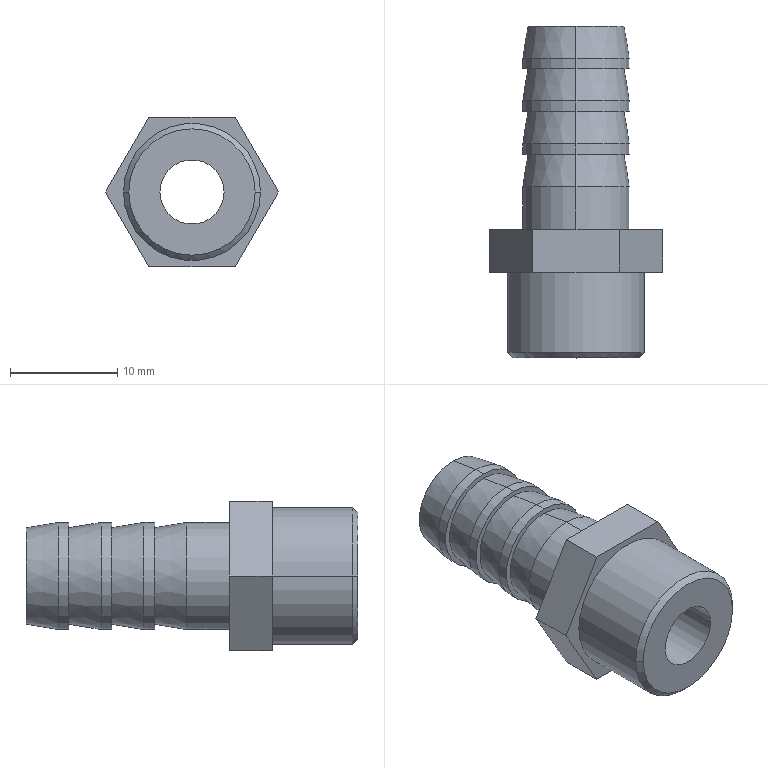Part | SolidWorks | features ICE 3, Chamfer 1, Revolution 1 | 1 solid | 35 faces | box 16.166 x 31 x 14 mm | volume 2228 mm3 | plane 13 | cylinder 12 | cone 10 | commonest cylinder face diameters 10 x8 6 x2 12.8 x2
STEP:
#1=CARTESIAN_POINT('',(5.9,-12.,0.));
#2=VERTEX_POINT('',#1);
#3=CARTESIAN_POINT('',(-5.9,-12.,0.));
#4=VERTEX_POINT('',#3);
#5=CARTESIAN_POINT('',(0.,-12.,0.));
#6=DIRECTION('',(0.,-1.,0.));
#7=DIRECTION('',(1.,0.,0.));
#8=AXIS2_PLACEMENT_3D('',#5,#6,#7);
#9=CIRCLE('',#8,5.9);
#10=EDGE_CURVE('',#2,#4,#9,.T.);
#11=ORIENTED_EDGE('',*,*,#10,.F.);
#12=CARTESIAN_POINT('',(6.4,-11.5,0.));
#13=VERTEX_POINT('',#12);
#14=CARTESIAN_POINT('',(5.9,-12.,0.));
#15=DIRECTION('',(0.7071,0.7071,0.));
#16=VECTOR('',#15,1000.);
#17=LINE('',#14,#16);
#18=EDGE_CURVE('',#2,#13,#17,.T.);
#19=ORIENTED_EDGE('',*,*,#18,.T.);
#20=CARTESIAN_POINT('',(-6.4,-11.5,0.));
#21=VERTEX_POINT('',#20);
#22=CARTESIAN_POINT('',(0.,-11.5,0.));
#23=DIRECTION('',(0.,1.,0.));
#24=DIRECTION('',(1.,0.,0.));
#25=AXIS2_PLACEMENT_3D('',#22,#23,#24);
#26=CIRCLE('',#25,6.4);
#27=EDGE_CURVE('',#21,#13,#26,.T.);
#28=ORIENTED_EDGE('',*,*,#27,.F.);
#29=CARTESIAN_POINT('',(-5.9,-12.,0.));
#30=DIRECTION('',(-0.7071,0.7071,0.));
#31=VECTOR('',#30,1000.);
#32=LINE('',#29,#31);
#33=EDGE_CURVE('',#4,#21,#32,.T.);
#34=ORIENTED_EDGE('',*,*,#33,.F.);
#35=EDGE_LOOP('',(#11,#19,#28,#34));
#36=FACE_OUTER_BOUND('',#35,.T.);
#37=CARTESIAN_POINT('',(0.,-12.,0.));
#38=DIRECTION('',(0.,1.,0.));
#39=DIRECTION('',(-1.,0.,0.));
#40=AXIS2_PLACEMENT_3D('',#37,#38,#39);
#41=CONICAL_SURFACE('',#40,5.9,0.7854);
#42=ADVANCED_FACE('',(#36),#41,.T.);
#43=CARTESIAN_POINT('',(3.,-12.,0.));
#44=VERTEX_POINT('',#43);
#45=CARTESIAN_POINT('',(-3.,-12.,0.));
#46=VERTEX_POINT('',#45);
#47=CARTESIAN_POINT('',(0.,-12.,0.));
#48=DIRECTION('',(0.,1.,0.));
#49=DIRECTION('',(1.,0.,0.));
#50=AXIS2_PLACEMENT_3D('',#47,#48,#49);
#51=CIRCLE('',#50,3.);
#52=EDGE_CURVE('',#44,#46,#51,.T.);
#53=ORIENTED_EDGE('',*,*,#52,.F.);
#54=CARTESIAN_POINT('',(3.,19.,0.));
#55=VERTEX_POINT('',#54);
#56=CARTESIAN_POINT('',(3.,-12.001,0.));
#57=DIRECTION('',(0.,1.,0.));
#58=VECTOR('',#57,1000.);
#59=LINE('',#56,#58);
#60=EDGE_CURVE('',#44,#55,#59,.T.);
#61=ORIENTED_EDGE('',*,*,#60,.T.);
#62=CARTESIAN_POINT('',(-3.,19.,0.));
#63=VERTEX_POINT('',#62);
#64=CARTESIAN_POINT('',(0.,19.,0.));
#65=DIRECTION('',(0.,1.,0.));
#66=DIRECTION('',(-1.,0.,0.));
#67=AXIS2_PLACEMENT_3D('',#64,#65,#66);
#68=CIRCLE('',#67,3.);
#69=EDGE_CURVE('',#55,#63,#68,.T.);
#70=ORIENTED_EDGE('',*,*,#69,.T.);
#71=CARTESIAN_POINT('',(-3.,-12.001,0.));
#72=DIRECTION('',(0.,1.,0.));
#73=VECTOR('',#72,1000.);
#74=LINE('',#71,#73);
#75=EDGE_CURVE('',#46,#63,#74,.T.);
#76=ORIENTED_EDGE('',*,*,#75,.F.);
#77=EDGE_LOOP('',(#53,#61,#70,#76));
#78=FACE_OUTER_BOUND('',#77,.T.);
#79=CARTESIAN_POINT('',(0.,-12.001,0.));
#80=DIRECTION('',(0.,1.,0.));
#81=DIRECTION('',(-1.,0.,0.));
#82=AXIS2_PLACEMENT_3D('',#79,#80,#81);
#83=CYLINDRICAL_SURFACE('',#82,3.);
#84=ADVANCED_FACE('',(#78),#83,.F.);
#85=ORIENTED_EDGE('',*,*,#27,.T.);
#86=CARTESIAN_POINT('',(6.4,-4.,0.));
#87=VERTEX_POINT('',#86);
#88=CARTESIAN_POINT('',(6.4,-12.,0.));
#89=DIRECTION('',(0.,1.,0.));
#90=VECTOR('',#89,1000.);
#91=LINE('',#88,#90);
#92=EDGE_CURVE('',#13,#87,#91,.T.);
#93=ORIENTED_EDGE('',*,*,#92,.T.);
#94=CARTESIAN_POINT('',(-6.4,-4.,0.));
#95=VERTEX_POINT('',#94);
#96=CARTESIAN_POINT('',(0.,-4.,0.));
#97=DIRECTION('',(0.,-1.,0.));
#98=DIRECTION('',(1.,0.,0.));
#99=AXIS2_PLACEMENT_3D('',#96,#97,#98);
#100=CIRCLE('',#99,6.4);
#101=EDGE_CURVE('',#87,#95,#100,.T.);
#102=ORIENTED_EDGE('',*,*,#101,.T.);
#103=CARTESIAN_POINT('',(-6.4,-12.,0.));
#104=DIRECTION('',(0.,1.,0.));
#105=VECTOR('',#104,1000.);
#106=LINE('',#103,#105);
#107=EDGE_CURVE('',#21,#95,#106,.T.);
#108=ORIENTED_EDGE('',*,*,#107,.F.);
#109=EDGE_LOOP('',(#85,#93,#102,#108));
#110=FACE_OUTER_BOUND('',#109,.T.);
#111=CARTESIAN_POINT('',(0.,-12.,0.));
#112=DIRECTION('',(0.,1.,0.));
#113=DIRECTION('',(-1.,0.,0.));
#114=AXIS2_PLACEMENT_3D('',#111,#112,#113);
#115=CYLINDRICAL_SURFACE('',#114,6.4);
#116=ADVANCED_FACE('',(#110),#115,.T.);
#117=CARTESIAN_POINT('',(0.,19.,-4.5));
#118=VERTEX_POINT('',#117);
#119=CARTESIAN_POINT('',(0.,19.,4.5));
#120=VERTEX_POINT('',#119);
#121=CARTESIAN_POINT('',(0.,19.,0.));
#122=DIRECTION('',(0.,-1.,0.));
#123=DIRECTION('',(0.,0.,-1.));
#124=AXIS2_PLACEMENT_3D('',#121,#122,#123);
#125=CIRCLE('',#124,4.5);
#126=EDGE_CURVE('',#118,#120,#125,.T.);
#127=ORIENTED_EDGE('',*,*,#126,.T.);
#128=CARTESIAN_POINT('',(0.,16.,5.));
#129=VERTEX_POINT('',#128);
#130=CARTESIAN_POINT('',(0.,19.,4.5));
#131=DIRECTION('',(0.,-0.9864,0.1644));
#132=VECTOR('',#131,1000.);
#133=LINE('',#130,#132);
#134=EDGE_CURVE('',#120,#129,#133,.T.);
#135=ORIENTED_EDGE('',*,*,#134,.T.);
#136=CARTESIAN_POINT('',(0.,16.,-5.));
#137=VERTEX_POINT('',#136);
#138=CARTESIAN_POINT('',(0.,16.,0.));
#139=DIRECTION('',(0.,-1.,0.));
#140=DIRECTION('',(0.,0.,-1.));
#141=AXIS2_PLACEMENT_3D('',#138,#139,#140);
#142=CIRCLE('',#141,5.);
#143=EDGE_CURVE('',#137,#129,#142,.T.);
#144=ORIENTED_EDGE('',*,*,#143,.F.);
#145=CARTESIAN_POINT('',(0.,19.,-4.5));
#146=DIRECTION('',(0.,-0.9864,-0.1644));
#147=VECTOR('',#146,1000.);
#148=LINE('',#145,#147);
#149=EDGE_CURVE('',#118,#137,#148,.T.);
#150=ORIENTED_EDGE('',*,*,#149,.F.);
#151=EDGE_LOOP('',(#127,#135,#144,#150));
#152=FACE_OUTER_BOUND('',#151,.T.);
#153=CARTESIAN_POINT('',(0.,19.,0.));
#154=DIRECTION('',(0.,-1.,0.));
#155=DIRECTION('',(0.,0.,-1.));
#156=AXIS2_PLACEMENT_3D('',#153,#154,#155);
#157=CONICAL_SURFACE('',#156,4.5,0.1651);
#158=ADVANCED_FACE('',(#152),#157,.T.);
#159=ORIENTED_EDGE('',*,*,#143,.T.);
#160=CARTESIAN_POINT('',(0.,15.,5.));
#161=VERTEX_POINT('',#160);
#162=CARTESIAN_POINT('',(0.,0.,5.));
#163=DIRECTION('',(0.,-1.,0.));
#164=VECTOR('',#163,1000.);
#165=LINE('',#162,#164);
#166=EDGE_CURVE('',#129,#161,#165,.T.);
#167=ORIENTED_EDGE('',*,*,#166,.T.);
#168=CARTESIAN_POINT('',(0.,15.,-5.));
#169=VERTEX_POINT('',#168);
#170=CARTESIAN_POINT('',(0.,15.,0.));
#171=DIRECTION('',(0.,-1.,0.));
#172=DIRECTION('',(0.,0.,-1.));
#173=AXIS2_PLACEMENT_3D('',#170,#171,#172);
#174=CIRCLE('',#173,5.);
#175=EDGE_CURVE('',#169,#161,#174,.T.);
#176=ORIENTED_EDGE('',*,*,#175,.F.);
#177=CARTESIAN_POINT('',(0.,0.,-5.));
#178=DIRECTION('',(0.,-1.,0.));
#179=VECTOR('',#178,1000.);
#180=LINE('',#177,#179);
#181=EDGE_CURVE('',#137,#169,#180,.T.);
#182=ORIENTED_EDGE('',*,*,#181,.F.);
#183=EDGE_LOOP('',(#159,#167,#176,#182));
#184=FACE_OUTER_BOUND('',#183,.T.);
#185=CARTESIAN_POINT('',(0.,0.,0.));
#186=DIRECTION('',(0.,-1.,0.));
#187=DIRECTION('',(0.,0.,-1.));
#188=AXIS2_PLACEMENT_3D('',#185,#186,#187);
#189=CYLINDRICAL_SURFACE('',#188,5.);
#190=ADVANCED_FACE('',(#184),#189,.T.);
#191=CARTESIAN_POINT('',(0.,15.,-4.5));
#192=VERTEX_POINT('',#191);
#193=CARTESIAN_POINT('',(0.,15.,4.5));
#194=VERTEX_POINT('',#193);
#195=CARTESIAN_POINT('',(0.,15.,0.));
#196=DIRECTION('',(0.,-1.,0.));
#197=DIRECTION('',(0.,0.,-1.));
#198=AXIS2_PLACEMENT_3D('',#195,#196,#197);
#199=CIRCLE('',#198,4.5);
#200=EDGE_CURVE('',#192,#194,#199,.T.);
#201=ORIENTED_EDGE('',*,*,#200,.T.);
#202=CARTESIAN_POINT('',(0.,12.,5.));
#203=VERTEX_POINT('',#202);
#204=CARTESIAN_POINT('',(0.,15.,4.5));
#205=DIRECTION('',(0.,-0.9864,0.1644));
#206=VECTOR('',#205,1000.);
#207=LINE('',#204,#206);
#208=EDGE_CURVE('',#194,#203,#207,.T.);
#209=ORIENTED_EDGE('',*,*,#208,.T.);
#210=CARTESIAN_POINT('',(0.,12.,-5.));
#211=VERTEX_POINT('',#210);
#212=CARTESIAN_POINT('',(0.,12.,0.));
#213=DIRECTION('',(0.,-1.,0.));
#214=DIRECTION('',(0.,0.,-1.));
#215=AXIS2_PLACEMENT_3D('',#212,#213,#214);
#216=CIRCLE('',#215,5.);
#217=EDGE_CURVE('',#211,#203,#216,.T.);
#218=ORIENTED_EDGE('',*,*,#217,.F.);
#219=CARTESIAN_POINT('',(0.,15.,-4.5));
#220=DIRECTION('',(0.,-0.9864,-0.1644));
#221=VECTOR('',#220,1000.);
#222=LINE('',#219,#221);
#223=EDGE_CURVE('',#192,#211,#222,.T.);
#224=ORIENTED_EDGE('',*,*,#223,.F.);
#225=EDGE_LOOP('',(#201,#209,#218,#224));
#226=FACE_OUTER_BOUND('',#225,.T.);
#227=CARTESIAN_POINT('',(0.,15.,0.));
#228=DIRECTION('',(0.,-1.,0.));
#229=DIRECTION('',(0.,0.,-1.));
#230=AXIS2_PLACEMENT_3D('',#227,#228,#229);
#231=CONICAL_SURFACE('',#230,4.5,0.1651);
#232=ADVANCED_FACE('',(#226),#231,.T.);
#233=ORIENTED_EDGE('',*,*,#217,.T.);
#234=CARTESIAN_POINT('',(0.,11.,5.));
#235=VERTEX_POINT('',#234);
#236=CARTESIAN_POINT('',(0.,0.,5.));
#237=DIRECTION('',(0.,-1.,0.));
#238=VECTOR('',#237,1000.);
#239=LINE('',#236,#238);
#240=EDGE_CURVE('',#203,#235,#239,.T.);
#241=ORIENTED_EDGE('',*,*,#240,.T.);
#242=CARTESIAN_POINT('',(0.,11.,-5.));
#243=VERTEX_POINT('',#242);
#244=CARTESIAN_POINT('',(0.,11.,0.));
#245=DIRECTION('',(0.,-1.,0.));
#246=DIRECTION('',(0.,0.,-1.));
#247=AXIS2_PLACEMENT_3D('',#244,#245,#246);
#248=CIRCLE('',#247,5.);
#249=EDGE_CURVE('',#243,#235,#248,.T.);
#250=ORIENTED_EDGE('',*,*,#249,.F.);
#251=CARTESIAN_POINT('',(0.,0.,-5.));
#252=DIRECTION('',(0.,-1.,0.));
#253=VECTOR('',#252,1000.);
#254=LINE('',#251,#253);
#255=EDGE_CURVE('',#211,#243,#254,.T.);
#256=ORIENTED_EDGE('',*,*,#255,.F.);
#257=EDGE_LOOP('',(#233,#241,#250,#256));
#258=FACE_OUTER_BOUND('',#257,.T.);
#259=CARTESIAN_POINT('',(0.,0.,0.));
#260=DIRECTION('',(0.,-1.,0.));
#261=DIRECTION('',(0.,0.,-1.));
#262=AXIS2_PLACEMENT_3D('',#259,#260,#261);
#263=CYLINDRICAL_SURFACE('',#262,5.);
#264=ADVANCED_FACE('',(#258),#263,.T.);
#265=CARTESIAN_POINT('',(0.,11.,-4.5));
#266=VERTEX_POINT('',#265);
#267=CARTESIAN_POINT('',(0.,11.,4.5));
#268=VERTEX_POINT('',#267);
#269=CARTESIAN_POINT('',(0.,11.,0.));
#270=DIRECTION('',(0.,-1.,0.));
#271=DIRECTION('',(0.,0.,-1.));
#272=AXIS2_PLACEMENT_3D('',#269,#270,#271);
#273=CIRCLE('',#272,4.5);
#274=EDGE_CURVE('',#266,#268,#273,.T.);
#275=ORIENTED_EDGE('',*,*,#274,.T.);
#276=CARTESIAN_POINT('',(0.,8.,5.));
#277=VERTEX_POINT('',#276);
#278=CARTESIAN_POINT('',(0.,11.,4.5));
#279=DIRECTION('',(0.,-0.9864,0.1644));
#280=VECTOR('',#279,1000.);
#281=LINE('',#278,#280);
#282=EDGE_CURVE('',#268,#277,#281,.T.);
#283=ORIENTED_EDGE('',*,*,#282,.T.);
#284=CARTESIAN_POINT('',(0.,8.,-5.));
#285=VERTEX_POINT('',#284);
#286=CARTESIAN_POINT('',(0.,8.,0.));
#287=DIRECTION('',(0.,-1.,0.));
#288=DIRECTION('',(0.,0.,-1.));
#289=AXIS2_PLACEMENT_3D('',#286,#287,#288);
#290=CIRCLE('',#289,5.);
#291=EDGE_CURVE('',#285,#277,#290,.T.);
#292=ORIENTED_EDGE('',*,*,#291,.F.);
#293=CARTESIAN_POINT('',(0.,11.,-4.5));
#294=DIRECTION('',(0.,-0.9864,-0.1644));
#295=VECTOR('',#294,1000.);
#296=LINE('',#293,#295);
#297=EDGE_CURVE('',#266,#285,#296,.T.);
#298=ORIENTED_EDGE('',*,*,#297,.F.);
#299=EDGE_LOOP('',(#275,#283,#292,#298));
#300=FACE_OUTER_BOUND('',#299,.T.);
#301=CARTESIAN_POINT('',(0.,11.,0.));
#302=DIRECTION('',(0.,-1.,0.));
#303=DIRECTION('',(0.,0.,-1.));
#304=AXIS2_PLACEMENT_3D('',#301,#302,#303);
#305=CONICAL_SURFACE('',#304,4.5,0.1651);
#306=ADVANCED_FACE('',(#300),#305,.T.);
#307=ORIENTED_EDGE('',*,*,#291,.T.);
#308=CARTESIAN_POINT('',(0.,7.,5.));
#309=VERTEX_POINT('',#308);
#310=CARTESIAN_POINT('',(0.,0.,5.));
#311=DIRECTION('',(0.,-1.,0.));
#312=VECTOR('',#311,1000.);
#313=LINE('',#310,#312);
#314=EDGE_CURVE('',#277,#309,#313,.T.);
#315=ORIENTED_EDGE('',*,*,#314,.T.);
#316=CARTESIAN_POINT('',(0.,7.,-5.));
#317=VERTEX_POINT('',#316);
#318=CARTESIAN_POINT('',(0.,7.,0.));
#319=DIRECTION('',(0.,-1.,0.));
#320=DIRECTION('',(0.,0.,-1.));
#321=AXIS2_PLACEMENT_3D('',#318,#319,#320);
#322=CIRCLE('',#321,5.);
#323=EDGE_CURVE('',#317,#309,#322,.T.);
#324=ORIENTED_EDGE('',*,*,#323,.F.);
#325=CARTESIAN_POINT('',(0.,0.,-5.));
#326=DIRECTION('',(0.,-1.,0.));
#327=VECTOR('',#326,1000.);
#328=LINE('',#325,#327);
#329=EDGE_CURVE('',#285,#317,#328,.T.);
#330=ORIENTED_EDGE('',*,*,#329,.F.);
#331=EDGE_LOOP('',(#307,#315,#324,#330));
#332=FACE_OUTER_BOUND('',#331,.T.);
#333=CARTESIAN_POINT('',(0.,0.,0.));
#334=DIRECTION('',(0.,-1.,0.));
#335=DIRECTION('',(0.,0.,-1.));
#336=AXIS2_PLACEMENT_3D('',#333,#334,#335);
#337=CYLINDRICAL_SURFACE('',#336,5.);
#338=ADVANCED_FACE('',(#332),#337,.T.);
#339=CARTESIAN_POINT('',(0.,7.,-4.5));
#340=VERTEX_POINT('',#339);
#341=CARTESIAN_POINT('',(0.,7.,4.5));
#342=VERTEX_POINT('',#341);
#343=CARTESIAN_POINT('',(0.,7.,0.));
#344=DIRECTION('',(0.,-1.,0.));
#345=DIRECTION('',(0.,0.,-1.));
#346=AXIS2_PLACEMENT_3D('',#343,#344,#345);
#347=CIRCLE('',#346,4.5);
#348=EDGE_CURVE('',#340,#342,#347,.T.);
#349=ORIENTED_EDGE('',*,*,#348,.T.);
#350=CARTESIAN_POINT('',(0.,4.,5.));
#351=VERTEX_POINT('',#350);
#352=CARTESIAN_POINT('',(0.,7.,4.5));
#353=DIRECTION('',(0.,-0.9864,0.1644));
#354=VECTOR('',#353,1000.);
#355=LINE('',#352,#354);
#356=EDGE_CURVE('',#342,#351,#355,.T.);
#357=ORIENTED_EDGE('',*,*,#356,.T.);
#358=CARTESIAN_POINT('',(0.,4.,-5.));
#359=VERTEX_POINT('',#358);
#360=CARTESIAN_POINT('',(0.,4.,0.));
#361=DIRECTION('',(0.,-1.,0.));
#362=DIRECTION('',(0.,0.,-1.));
#363=AXIS2_PLACEMENT_3D('',#360,#361,#362);
#364=CIRCLE('',#363,5.);
#365=EDGE_CURVE('',#359,#351,#364,.T.);
#366=ORIENTED_EDGE('',*,*,#365,.F.);
#367=CARTESIAN_POINT('',(0.,7.,-4.5));
#368=DIRECTION('',(0.,-0.9864,-0.1644));
#369=VECTOR('',#368,1000.);
#370=LINE('',#367,#369);
#371=EDGE_CURVE('',#340,#359,#370,.T.);
#372=ORIENTED_EDGE('',*,*,#371,.F.);
#373=EDGE_LOOP('',(#349,#357,#366,#372));
#374=FACE_OUTER_BOUND('',#373,.T.);
#375=CARTESIAN_POINT('',(0.,7.,0.));
#376=DIRECTION('',(0.,-1.,0.));
#377=DIRECTION('',(0.,0.,-1.));
#378=AXIS2_PLACEMENT_3D('',#375,#376,#377);
#379=CONICAL_SURFACE('',#378,4.5,0.1651);
#380=ADVANCED_FACE('',(#374),#379,.T.);
#381=ORIENTED_EDGE('',*,*,#365,.T.);
#382=CARTESIAN_POINT('',(0.,0.,5.));
#383=VERTEX_POINT('',#382);
#384=CARTESIAN_POINT('',(0.,0.,5.));
#385=DIRECTION('',(0.,-1.,0.));
#386=VECTOR('',#385,1000.);
#387=LINE('',#384,#386);
#388=EDGE_CURVE('',#351,#383,#387,.T.);
#389=ORIENTED_EDGE('',*,*,#388,.T.);
#390=CARTESIAN_POINT('',(0.,0.,-5.));
#391=VERTEX_POINT('',#390);
#392=CARTESIAN_POINT('',(0.,0.,0.));
#393=DIRECTION('',(0.,-1.,0.));
#394=DIRECTION('',(0.,0.,-1.));
#395=AXIS2_PLACEMENT_3D('',#392,#393,#394);
#396=CIRCLE('',#395,5.);
#397=EDGE_CURVE('',#391,#383,#396,.T.);
#398=ORIENTED_EDGE('',*,*,#397,.F.);
#399=CARTESIAN_POINT('',(0.,0.,-5.));
#400=DIRECTION('',(0.,-1.,0.));
#401=VECTOR('',#400,1000.);
#402=LINE('',#399,#401);
#403=EDGE_CURVE('',#359,#391,#402,.T.);
#404=ORIENTED_EDGE('',*,*,#403,.F.);
#405=EDGE_LOOP('',(#381,#389,#398,#404));
#406=FACE_OUTER_BOUND('',#405,.T.);
#407=CARTESIAN_POINT('',(0.,0.,0.));
#408=DIRECTION('',(0.,-1.,0.));
#409=DIRECTION('',(0.,0.,-1.));
#410=AXIS2_PLACEMENT_3D('',#407,#408,#409);
#411=CYLINDRICAL_SURFACE('',#410,5.);
#412=ADVANCED_FACE('',(#406),#411,.T.);
#413=ORIENTED_EDGE('',*,*,#388,.F.);
#414=CARTESIAN_POINT('',(0.,4.,0.));
#415=DIRECTION('',(0.,-1.,0.));
#416=DIRECTION('',(0.,0.,-1.));
#417=AXIS2_PLACEMENT_3D('',#414,#415,#416);
#418=CIRCLE('',#417,5.);
#419=EDGE_CURVE('',#351,#359,#418,.T.);
#420=ORIENTED_EDGE('',*,*,#419,.T.);
#421=ORIENTED_EDGE('',*,*,#403,.T.);
#422=CARTESIAN_POINT('',(0.,0.,0.));
#423=DIRECTION('',(0.,-1.,0.));
#424=DIRECTION('',(0.,0.,-1.));
#425=AXIS2_PLACEMENT_3D('',#422,#423,#424);
#426=CIRCLE('',#425,5.);
#427=EDGE_CURVE('',#383,#391,#426,.T.);
#428=ORIENTED_EDGE('',*,*,#427,.F.);
#429=EDGE_LOOP('',(#413,#420,#421,#428));
#430=FACE_OUTER_BOUND('',#429,.T.);
#431=CARTESIAN_POINT('',(0.,0.,0.));
#432=DIRECTION('',(0.,-1.,0.));
#433=DIRECTION('',(0.,0.,-1.));
#434=AXIS2_PLACEMENT_3D('',#431,#432,#433);
#435=CYLINDRICAL_SURFACE('',#434,5.);
#436=ADVANCED_FACE('',(#430),#435,.T.);
#437=ORIENTED_EDGE('',*,*,#356,.F.);
#438=CARTESIAN_POINT('',(0.,7.,0.));
#439=DIRECTION('',(0.,-1.,0.));
#440=DIRECTION('',(0.,0.,-1.));
#441=AXIS2_PLACEMENT_3D('',#438,#439,#440);
#442=CIRCLE('',#441,4.5);
#443=EDGE_CURVE('',#342,#340,#442,.T.);
#444=ORIENTED_EDGE('',*,*,#443,.T.);
#445=ORIENTED_EDGE('',*,*,#371,.T.);
#446=ORIENTED_EDGE('',*,*,#419,.F.);
#447=EDGE_LOOP('',(#437,#444,#445,#446));
#448=FACE_OUTER_BOUND('',#447,.T.);
#449=CARTESIAN_POINT('',(0.,7.,0.));
#450=DIRECTION('',(0.,-1.,0.));
#451=DIRECTION('',(0.,0.,-1.));
#452=AXIS2_PLACEMENT_3D('',#449,#450,#451);
#453=CONICAL_SURFACE('',#452,4.5,0.1651);
#454=ADVANCED_FACE('',(#448),#453,.T.);
#455=ORIENTED_EDGE('',*,*,#348,.F.);
#456=ORIENTED_EDGE('',*,*,#443,.F.);
#457=EDGE_LOOP('',(#455,#456));
#458=FACE_BOUND('',#457,.T.);
#459=ORIENTED_EDGE('',*,*,#323,.T.);
#460=CARTESIAN_POINT('',(0.,7.,0.));
#461=DIRECTION('',(0.,-1.,0.));
#462=DIRECTION('',(0.,0.,-1.));
#463=AXIS2_PLACEMENT_3D('',#460,#461,#462);
#464=CIRCLE('',#463,5.);
#465=EDGE_CURVE('',#309,#317,#464,.T.);
#466=ORIENTED_EDGE('',*,*,#465,.T.);
#467=EDGE_LOOP('',(#459,#466));
#468=FACE_OUTER_BOUND('',#467,.T.);
#469=CARTESIAN_POINT('',(-5.,7.,0.));
#470=DIRECTION('',(0.,1.,0.));
#471=DIRECTION('',(0.,0.,1.));
#472=AXIS2_PLACEMENT_3D('',#469,#470,#471);
#473=PLANE('',#472);
#474=ADVANCED_FACE('',(#458,#468),#473,.F.);
#475=ORIENTED_EDGE('',*,*,#314,.F.);
#476=CARTESIAN_POINT('',(0.,8.,0.));
#477=DIRECTION('',(0.,-1.,0.));
#478=DIRECTION('',(0.,0.,-1.));
#479=AXIS2_PLACEMENT_3D('',#476,#477,#478);
#480=CIRCLE('',#479,5.);
#481=EDGE_CURVE('',#277,#285,#480,.T.);
#482=ORIENTED_EDGE('',*,*,#481,.T.);
#483=ORIENTED_EDGE('',*,*,#329,.T.);
#484=ORIENTED_EDGE('',*,*,#465,.F.);
#485=EDGE_LOOP('',(#475,#482,#483,#484));
#486=FACE_OUTER_BOUND('',#485,.T.);
#487=CARTESIAN_POINT('',(0.,0.,0.));
#488=DIRECTION('',(0.,-1.,0.));
#489=DIRECTION('',(0.,0.,-1.));
#490=AXIS2_PLACEMENT_3D('',#487,#488,#489);
#491=CYLINDRICAL_SURFACE('',#490,5.);
#492=ADVANCED_FACE('',(#486),#491,.T.);
#493=ORIENTED_EDGE('',*,*,#282,.F.);
#494=CARTESIAN_POINT('',(0.,11.,0.));
#495=DIRECTION('',(0.,-1.,0.));
#496=DIRECTION('',(0.,0.,-1.));
#497=AXIS2_PLACEMENT_3D('',#494,#495,#496);
#498=CIRCLE('',#497,4.5);
#499=EDGE_CURVE('',#268,#266,#498,.T.);
#500=ORIENTED_EDGE('',*,*,#499,.T.);
#501=ORIENTED_EDGE('',*,*,#297,.T.);
#502=ORIENTED_EDGE('',*,*,#481,.F.);
#503=EDGE_LOOP('',(#493,#500,#501,#502));
#504=FACE_OUTER_BOUND('',#503,.T.);
#505=CARTESIAN_POINT('',(0.,11.,0.));
#506=DIRECTION('',(0.,-1.,0.));
#507=DIRECTION('',(0.,0.,-1.));
#508=AXIS2_PLACEMENT_3D('',#505,#506,#507);
#509=CONICAL_SURFACE('',#508,4.5,0.1651);
#510=ADVANCED_FACE('',(#504),#509,.T.);
#511=ORIENTED_EDGE('',*,*,#274,.F.);
#512=ORIENTED_EDGE('',*,*,#499,.F.);
#513=EDGE_LOOP('',(#511,#512));
#514=FACE_BOUND('',#513,.T.);
#515=ORIENTED_EDGE('',*,*,#249,.T.);
#516=CARTESIAN_POINT('',(0.,11.,0.));
#517=DIRECTION('',(0.,-1.,0.));
#518=DIRECTION('',(0.,0.,-1.));
#519=AXIS2_PLACEMENT_3D('',#516,#517,#518);
#520=CIRCLE('',#519,5.);
#521=EDGE_CURVE('',#235,#243,#520,.T.);
#522=ORIENTED_EDGE('',*,*,#521,.T.);
#523=EDGE_LOOP('',(#515,#522));
#524=FACE_OUTER_BOUND('',#523,.T.);
#525=CARTESIAN_POINT('',(-5.,11.,0.));
#526=DIRECTION('',(0.,1.,0.));
#527=DIRECTION('',(0.,0.,1.));
#528=AXIS2_PLACEMENT_3D('',#525,#526,#527);
#529=PLANE('',#528);
#530=ADVANCED_FACE('',(#514,#524),#529,.F.);
#531=ORIENTED_EDGE('',*,*,#240,.F.);
#532=CARTESIAN_POINT('',(0.,12.,0.));
#533=DIRECTION('',(0.,-1.,0.));
#534=DIRECTION('',(0.,0.,-1.));
#535=AXIS2_PLACEMENT_3D('',#532,#533,#534);
#536=CIRCLE('',#535,5.);
#537=EDGE_CURVE('',#203,#211,#536,.T.);
#538=ORIENTED_EDGE('',*,*,#537,.T.);
#539=ORIENTED_EDGE('',*,*,#255,.T.);
#540=ORIENTED_EDGE('',*,*,#521,.F.);
#541=EDGE_LOOP('',(#531,#538,#539,#540));
#542=FACE_OUTER_BOUND('',#541,.T.);
#543=CARTESIAN_POINT('',(0.,0.,0.));
#544=DIRECTION('',(0.,-1.,0.));
#545=DIRECTION('',(0.,0.,-1.));
#546=AXIS2_PLACEMENT_3D('',#543,#544,#545);
#547=CYLINDRICAL_SURFACE('',#546,5.);
#548=ADVANCED_FACE('',(#542),#547,.T.);
#549=ORIENTED_EDGE('',*,*,#208,.F.);
#550=CARTESIAN_POINT('',(0.,15.,0.));
#551=DIRECTION('',(0.,-1.,0.));
#552=DIRECTION('',(0.,0.,-1.));
#553=AXIS2_PLACEMENT_3D('',#550,#551,#552);
#554=CIRCLE('',#553,4.5);
#555=EDGE_CURVE('',#194,#192,#554,.T.);
#556=ORIENTED_EDGE('',*,*,#555,.T.);
#557=ORIENTED_EDGE('',*,*,#223,.T.);
#558=ORIENTED_EDGE('',*,*,#537,.F.);
#559=EDGE_LOOP('',(#549,#556,#557,#558));
#560=FACE_OUTER_BOUND('',#559,.T.);
#561=CARTESIAN_POINT('',(0.,15.,0.));
#562=DIRECTION('',(0.,-1.,0.));
#563=DIRECTION('',(0.,0.,-1.));
#564=AXIS2_PLACEMENT_3D('',#561,#562,#563);
#565=CONICAL_SURFACE('',#564,4.5,0.1651);
#566=ADVANCED_FACE('',(#560),#565,.T.);
#567=ORIENTED_EDGE('',*,*,#200,.F.);
#568=ORIENTED_EDGE('',*,*,#555,.F.);
#569=EDGE_LOOP('',(#567,#568));
#570=FACE_BOUND('',#569,.T.);
#571=ORIENTED_EDGE('',*,*,#175,.T.);
#572=CARTESIAN_POINT('',(0.,15.,0.));
#573=DIRECTION('',(0.,-1.,0.));
#574=DIRECTION('',(0.,0.,-1.));
#575=AXIS2_PLACEMENT_3D('',#572,#573,#574);
#576=CIRCLE('',#575,5.);
#577=EDGE_CURVE('',#161,#169,#576,.T.);
#578=ORIENTED_EDGE('',*,*,#577,.T.);
#579=EDGE_LOOP('',(#571,#578));
#580=FACE_OUTER_BOUND('',#579,.T.);
#581=CARTESIAN_POINT('',(-5.,15.,0.));
#582=DIRECTION('',(0.,1.,0.));
#583=DIRECTION('',(0.,0.,1.));
#584=AXIS2_PLACEMENT_3D('',#581,#582,#583);
#585=PLANE('',#584);
#586=ADVANCED_FACE('',(#570,#580),#585,.F.);
#587=ORIENTED_EDGE('',*,*,#166,.F.);
#588=CARTESIAN_POINT('',(0.,16.,0.));
#589=DIRECTION('',(0.,-1.,0.));
#590=DIRECTION('',(0.,0.,-1.));
#591=AXIS2_PLACEMENT_3D('',#588,#589,#590);
#592=CIRCLE('',#591,5.);
#593=EDGE_CURVE('',#129,#137,#592,.T.);
#594=ORIENTED_EDGE('',*,*,#593,.T.);
#595=ORIENTED_EDGE('',*,*,#181,.T.);
#596=ORIENTED_EDGE('',*,*,#577,.F.);
#597=EDGE_LOOP('',(#587,#594,#595,#596));
#598=FACE_OUTER_BOUND('',#597,.T.);
#599=CARTESIAN_POINT('',(0.,0.,0.));
#600=DIRECTION('',(0.,-1.,0.));
#601=DIRECTION('',(0.,0.,-1.));
#602=AXIS2_PLACEMENT_3D('',#599,#600,#601);
#603=CYLINDRICAL_SURFACE('',#602,5.);
#604=ADVANCED_FACE('',(#598),#603,.T.);
#605=ORIENTED_EDGE('',*,*,#134,.F.);
#606=CARTESIAN_POINT('',(0.,19.,0.));
#607=DIRECTION('',(0.,-1.,0.));
#608=DIRECTION('',(0.,0.,-1.));
#609=AXIS2_PLACEMENT_3D('',#606,#607,#608);
#610=CIRCLE('',#609,4.5);
#611=EDGE_CURVE('',#120,#118,#610,.T.);
#612=ORIENTED_EDGE('',*,*,#611,.T.);
#613=ORIENTED_EDGE('',*,*,#149,.T.);
#614=ORIENTED_EDGE('',*,*,#593,.F.);
#615=EDGE_LOOP('',(#605,#612,#613,#614));
#616=FACE_OUTER_BOUND('',#615,.T.);
#617=CARTESIAN_POINT('',(0.,19.,0.));
#618=DIRECTION('',(0.,-1.,0.));
#619=DIRECTION('',(0.,0.,-1.));
#620=AXIS2_PLACEMENT_3D('',#617,#618,#619);
#621=CONICAL_SURFACE('',#620,4.5,0.1651);
#622=ADVANCED_FACE('',(#616),#621,.T.);
#623=CARTESIAN_POINT('',(0.,19.,0.));
#624=DIRECTION('',(0.,1.,0.));
#625=DIRECTION('',(-1.,0.,0.));
#626=AXIS2_PLACEMENT_3D('',#623,#624,#625);
#627=CIRCLE('',#626,3.);
#628=EDGE_CURVE('',#63,#55,#627,.T.);
#629=ORIENTED_EDGE('',*,*,#628,.F.);
#630=ORIENTED_EDGE('',*,*,#69,.F.);
#631=EDGE_LOOP('',(#629,#630));
#632=FACE_BOUND('',#631,.T.);
#633=ORIENTED_EDGE('',*,*,#126,.F.);
#634=ORIENTED_EDGE('',*,*,#611,.F.);
#635=EDGE_LOOP('',(#633,#634));
#636=FACE_OUTER_BOUND('',#635,.T.);
#637=CARTESIAN_POINT('',(-4.5,19.,0.));
#638=DIRECTION('',(0.,-1.,0.));
#639=DIRECTION('',(0.,0.,-1.));
#640=AXIS2_PLACEMENT_3D('',#637,#638,#639);
#641=PLANE('',#640);
#642=ADVANCED_FACE('',(#632,#636),#641,.F.);
#643=CARTESIAN_POINT('',(4.041,0.,-7.));
#644=VERTEX_POINT('',#643);
#645=CARTESIAN_POINT('',(8.083,0.,0.));
#646=VERTEX_POINT('',#645);
#647=CARTESIAN_POINT('',(4.041,0.,-7.));
#648=DIRECTION('',(0.5,0.,0.866));
#649=VECTOR('',#648,1000.);
#650=LINE('',#647,#649);
#651=EDGE_CURVE('',#644,#646,#650,.T.);
#652=ORIENTED_EDGE('',*,*,#651,.T.);
#653=CARTESIAN_POINT('',(8.083,-4.,0.));
#654=VERTEX_POINT('',#653);
#655=CARTESIAN_POINT('',(8.083,-4.,0.));
#656=DIRECTION('',(0.,1.,0.));
#657=VECTOR('',#656,1000.);
#658=LINE('',#655,#657);
#659=EDGE_CURVE('',#654,#646,#658,.T.);
#660=ORIENTED_EDGE('',*,*,#659,.F.);
#661=CARTESIAN_POINT('',(4.041,-4.,-7.));
#662=VERTEX_POINT('',#661);
#663=CARTESIAN_POINT('',(4.041,-4.,-7.));
#664=DIRECTION('',(0.5,0.,0.866));
#665=VECTOR('',#664,1000.);
#666=LINE('',#663,#665);
#667=EDGE_CURVE('',#662,#654,#666,.T.);
#668=ORIENTED_EDGE('',*,*,#667,.F.);
#669=CARTESIAN_POINT('',(4.041,-4.,-7.));
#670=DIRECTION('',(0.,1.,0.));
#671=VECTOR('',#670,1000.);
#672=LINE('',#669,#671);
#673=EDGE_CURVE('',#662,#644,#672,.T.);
#674=ORIENTED_EDGE('',*,*,#673,.T.);
#675=EDGE_LOOP('',(#652,#660,#668,#674));
#676=FACE_OUTER_BOUND('',#675,.T.);
#677=CARTESIAN_POINT('',(4.041,-4.,-7.));
#678=DIRECTION('',(-0.866,0.,0.5));
#679=DIRECTION('',(0.5,0.,0.866));
#680=AXIS2_PLACEMENT_3D('',#677,#678,#679);
#681=PLANE('',#680);
#682=ADVANCED_FACE('',(#676),#681,.F.);
#683=CARTESIAN_POINT('',(4.041,0.,7.));
#684=VERTEX_POINT('',#683);
#685=CARTESIAN_POINT('',(8.083,0.,0.));
#686=DIRECTION('',(-0.5,0.,0.866));
#687=VECTOR('',#686,1000.);
#688=LINE('',#685,#687);
#689=EDGE_CURVE('',#646,#684,#688,.T.);
#690=ORIENTED_EDGE('',*,*,#689,.T.);
#691=CARTESIAN_POINT('',(4.041,-4.,7.));
#692=VERTEX_POINT('',#691);
#693=CARTESIAN_POINT('',(4.041,-4.,7.));
#694=DIRECTION('',(0.,1.,0.));
#695=VECTOR('',#694,1000.);
#696=LINE('',#693,#695);
#697=EDGE_CURVE('',#692,#684,#696,.T.);
#698=ORIENTED_EDGE('',*,*,#697,.F.);
#699=CARTESIAN_POINT('',(8.083,-4.,0.));
#700=DIRECTION('',(-0.5,0.,0.866));
#701=VECTOR('',#700,1000.);
#702=LINE('',#699,#701);
#703=EDGE_CURVE('',#654,#692,#702,.T.);
#704=ORIENTED_EDGE('',*,*,#703,.F.);
#705=ORIENTED_EDGE('',*,*,#659,.T.);
#706=EDGE_LOOP('',(#690,#698,#704,#705));
#707=FACE_OUTER_BOUND('',#706,.T.);
#708=CARTESIAN_POINT('',(8.083,-4.,0.));
#709=DIRECTION('',(-0.866,0.,-0.5));
#710=DIRECTION('',(-0.5,0.,0.866));
#711=AXIS2_PLACEMENT_3D('',#708,#709,#710);
#712=PLANE('',#711);
#713=ADVANCED_FACE('',(#707),#712,.F.);
#714=CARTESIAN_POINT('',(-4.041,0.,7.));
#715=VERTEX_POINT('',#714);
#716=CARTESIAN_POINT('',(4.041,0.,7.));
#717=DIRECTION('',(-1.,0.,0.));
#718=VECTOR('',#717,1000.);
#719=LINE('',#716,#718);
#720=EDGE_CURVE('',#684,#715,#719,.T.);
#721=ORIENTED_EDGE('',*,*,#720,.T.);
#722=CARTESIAN_POINT('',(-4.041,-4.,7.));
#723=VERTEX_POINT('',#722);
#724=CARTESIAN_POINT('',(-4.041,-4.,7.));
#725=DIRECTION('',(0.,1.,0.));
#726=VECTOR('',#725,1000.);
#727=LINE('',#724,#726);
#728=EDGE_CURVE('',#723,#715,#727,.T.);
#729=ORIENTED_EDGE('',*,*,#728,.F.);
#730=CARTESIAN_POINT('',(4.041,-4.,7.));
#731=DIRECTION('',(-1.,0.,0.));
#732=VECTOR('',#731,1000.);
#733=LINE('',#730,#732);
#734=EDGE_CURVE('',#692,#723,#733,.T.);
#735=ORIENTED_EDGE('',*,*,#734,.F.);
#736=ORIENTED_EDGE('',*,*,#697,.T.);
#737=EDGE_LOOP('',(#721,#729,#735,#736));
#738=FACE_OUTER_BOUND('',#737,.T.);
#739=CARTESIAN_POINT('',(4.041,-4.,7.));
#740=DIRECTION('',(0.,0.,-1.));
#741=DIRECTION('',(-1.,0.,0.));
#742=AXIS2_PLACEMENT_3D('',#739,#740,#741);
#743=PLANE('',#742);
#744=ADVANCED_FACE('',(#738),#743,.F.);
#745=CARTESIAN_POINT('',(-8.083,0.,0.));
#746=VERTEX_POINT('',#745);
#747=CARTESIAN_POINT('',(-4.041,0.,7.));
#748=DIRECTION('',(-0.5,0.,-0.866));
#749=VECTOR('',#748,1000.);
#750=LINE('',#747,#749);
#751=EDGE_CURVE('',#715,#746,#750,.T.);
#752=ORIENTED_EDGE('',*,*,#751,.T.);
#753=CARTESIAN_POINT('',(-8.083,-4.,0.));
#754=VERTEX_POINT('',#753);
#755=CARTESIAN_POINT('',(-8.083,-4.,0.));
#756=DIRECTION('',(0.,1.,0.));
#757=VECTOR('',#756,1000.);
#758=LINE('',#755,#757);
#759=EDGE_CURVE('',#754,#746,#758,.T.);
#760=ORIENTED_EDGE('',*,*,#759,.F.);
#761=CARTESIAN_POINT('',(-4.041,-4.,7.));
#762=DIRECTION('',(-0.5,0.,-0.866));
#763=VECTOR('',#762,1000.);
#764=LINE('',#761,#763);
#765=EDGE_CURVE('',#723,#754,#764,.T.);
#766=ORIENTED_EDGE('',*,*,#765,.F.);
#767=ORIENTED_EDGE('',*,*,#728,.T.);
#768=EDGE_LOOP('',(#752,#760,#766,#767));
#769=FACE_OUTER_BOUND('',#768,.T.);
#770=CARTESIAN_POINT('',(-4.041,-4.,7.));
#771=DIRECTION('',(0.866,0.,-0.5));
#772=DIRECTION('',(-0.5,0.,-0.866));
#773=AXIS2_PLACEMENT_3D('',#770,#771,#772);
#774=PLANE('',#773);
#775=ADVANCED_FACE('',(#769),#774,.F.);
#776=CARTESIAN_POINT('',(-4.041,0.,-7.));
#777=VERTEX_POINT('',#776);
#778=CARTESIAN_POINT('',(-8.083,0.,0.));
#779=DIRECTION('',(0.5,0.,-0.866));
#780=VECTOR('',#779,1000.);
#781=LINE('',#778,#780);
#782=EDGE_CURVE('',#746,#777,#781,.T.);
#783=ORIENTED_EDGE('',*,*,#782,.T.);
#784=CARTESIAN_POINT('',(-4.041,-4.,-7.));
#785=VERTEX_POINT('',#784);
#786=CARTESIAN_POINT('',(-4.041,-4.,-7.));
#787=DIRECTION('',(0.,1.,0.));
#788=VECTOR('',#787,1000.);
#789=LINE('',#786,#788);
#790=EDGE_CURVE('',#785,#777,#789,.T.);
#791=ORIENTED_EDGE('',*,*,#790,.F.);
#792=CARTESIAN_POINT('',(-8.083,-4.,0.));
#793=DIRECTION('',(0.5,0.,-0.866));
#794=VECTOR('',#793,1000.);
#795=LINE('',#792,#794);
#796=EDGE_CURVE('',#754,#785,#795,.T.);
#797=ORIENTED_EDGE('',*,*,#796,.F.);
#798=ORIENTED_EDGE('',*,*,#759,.T.);
#799=EDGE_LOOP('',(#783,#791,#797,#798));
#800=FACE_OUTER_BOUND('',#799,.T.);
#801=CARTESIAN_POINT('',(-8.083,-4.,0.));
#802=DIRECTION('',(0.866,0.,0.5));
#803=DIRECTION('',(0.5,0.,-0.866));
#804=AXIS2_PLACEMENT_3D('',#801,#802,#803);
#805=PLANE('',#804);
#806=ADVANCED_FACE('',(#800),#805,.F.);
#807=CARTESIAN_POINT('',(-4.041,0.,-7.));
#808=DIRECTION('',(1.,0.,0.));
#809=VECTOR('',#808,1000.);
#810=LINE('',#807,#809);
#811=EDGE_CURVE('',#777,#644,#810,.T.);
#812=ORIENTED_EDGE('',*,*,#811,.T.);
#813=ORIENTED_EDGE('',*,*,#673,.F.);
#814=CARTESIAN_POINT('',(-4.041,-4.,-7.));
#815=DIRECTION('',(1.,0.,0.));
#816=VECTOR('',#815,1000.);
#817=LINE('',#814,#816);
#818=EDGE_CURVE('',#785,#662,#817,.T.);
#819=ORIENTED_EDGE('',*,*,#818,.F.);
#820=ORIENTED_EDGE('',*,*,#790,.T.);
#821=EDGE_LOOP('',(#812,#813,#819,#820));
#822=FACE_OUTER_BOUND('',#821,.T.);
#823=CARTESIAN_POINT('',(-4.041,-4.,-7.));
#824=DIRECTION('',(0.,0.,1.));
#825=DIRECTION('',(1.,0.,0.));
#826=AXIS2_PLACEMENT_3D('',#823,#824,#825);
#827=PLANE('',#826);
#828=ADVANCED_FACE('',(#822),#827,.F.);
#829=CARTESIAN_POINT('',(0.,-4.,0.));
#830=DIRECTION('',(0.,-1.,0.));
#831=DIRECTION('',(1.,0.,0.));
#832=AXIS2_PLACEMENT_3D('',#829,#830,#831);
#833=CIRCLE('',#832,6.4);
#834=EDGE_CURVE('',#95,#87,#833,.T.);
#835=ORIENTED_EDGE('',*,*,#834,.F.);
#836=ORIENTED_EDGE('',*,*,#101,.F.);
#837=EDGE_LOOP('',(#835,#836));
#838=FACE_BOUND('',#837,.T.);
#839=ORIENTED_EDGE('',*,*,#667,.T.);
#840=ORIENTED_EDGE('',*,*,#703,.T.);
#841=ORIENTED_EDGE('',*,*,#734,.T.);
#842=ORIENTED_EDGE('',*,*,#765,.T.);
#843=ORIENTED_EDGE('',*,*,#796,.T.);
#844=ORIENTED_EDGE('',*,*,#818,.T.);
#845=EDGE_LOOP('',(#839,#840,#841,#842,#843,#844));
#846=FACE_OUTER_BOUND('',#845,.T.);
#847=CARTESIAN_POINT('',(0.,-4.,0.));
#848=DIRECTION('',(0.,-1.,0.));
#849=DIRECTION('',(1.,0.,0.));
#850=AXIS2_PLACEMENT_3D('',#847,#848,#849);
#851=PLANE('',#850);
#852=ADVANCED_FACE('',(#838,#846),#851,.T.);
#853=ORIENTED_EDGE('',*,*,#397,.T.);
#854=ORIENTED_EDGE('',*,*,#427,.T.);
#855=EDGE_LOOP('',(#853,#854));
#856=FACE_BOUND('',#855,.T.);
#857=ORIENTED_EDGE('',*,*,#651,.F.);
#858=ORIENTED_EDGE('',*,*,#811,.F.);
#859=ORIENTED_EDGE('',*,*,#782,.F.);
#860=ORIENTED_EDGE('',*,*,#751,.F.);
#861=ORIENTED_EDGE('',*,*,#720,.F.);
#862=ORIENTED_EDGE('',*,*,#689,.F.);
#863=EDGE_LOOP('',(#857,#858,#859,#860,#861,#862));
#864=FACE_OUTER_BOUND('',#863,.T.);
#865=CARTESIAN_POINT('',(0.,0.,0.));
#866=DIRECTION('',(0.,-1.,0.));
#867=DIRECTION('',(1.,0.,0.));
#868=AXIS2_PLACEMENT_3D('',#865,#866,#867);
#869=PLANE('',#868);
#870=ADVANCED_FACE('',(#856,#864),#869,.F.);
#871=ORIENTED_EDGE('',*,*,#92,.F.);
#872=CARTESIAN_POINT('',(0.,-11.5,0.));
#873=DIRECTION('',(0.,1.,0.));
#874=DIRECTION('',(1.,0.,0.));
#875=AXIS2_PLACEMENT_3D('',#872,#873,#874);
#876=CIRCLE('',#875,6.4);
#877=EDGE_CURVE('',#13,#21,#876,.T.);
#878=ORIENTED_EDGE('',*,*,#877,.T.);
#879=ORIENTED_EDGE('',*,*,#107,.T.);
#880=ORIENTED_EDGE('',*,*,#834,.T.);
#881=EDGE_LOOP('',(#871,#878,#879,#880));
#882=FACE_OUTER_BOUND('',#881,.T.);
#883=CARTESIAN_POINT('',(0.,-12.,0.));
#884=DIRECTION('',(0.,1.,0.));
#885=DIRECTION('',(-1.,0.,0.));
#886=AXIS2_PLACEMENT_3D('',#883,#884,#885);
#887=CYLINDRICAL_SURFACE('',#886,6.4);
#888=ADVANCED_FACE('',(#882),#887,.T.);
#889=CARTESIAN_POINT('',(0.,-12.,0.));
#890=DIRECTION('',(0.,-1.,0.));
#891=DIRECTION('',(1.,0.,0.));
#892=AXIS2_PLACEMENT_3D('',#889,#890,#891);
#893=CIRCLE('',#892,5.9);
#894=EDGE_CURVE('',#4,#2,#893,.T.);
#895=ORIENTED_EDGE('',*,*,#894,.T.);
#896=ORIENTED_EDGE('',*,*,#10,.T.);
#897=EDGE_LOOP('',(#895,#896));
#898=FACE_OUTER_BOUND('',#897,.T.);
#899=CARTESIAN_POINT('',(0.,-12.,0.));
#900=DIRECTION('',(0.,1.,0.));
#901=DIRECTION('',(1.,0.,0.));
#902=AXIS2_PLACEMENT_3D('',#899,#900,#901);
#903=CIRCLE('',#902,3.);
#904=EDGE_CURVE('',#46,#44,#903,.T.);
#905=ORIENTED_EDGE('',*,*,#904,.T.);
#906=ORIENTED_EDGE('',*,*,#52,.T.);
#907=EDGE_LOOP('',(#905,#906));
#908=FACE_BOUND('',#907,.T.);
#909=CARTESIAN_POINT('',(0.,-12.,0.));
#910=DIRECTION('',(0.,-1.,0.));
#911=DIRECTION('',(1.,0.,0.));
#912=AXIS2_PLACEMENT_3D('',#909,#910,#911);
#913=PLANE('',#912);
#914=ADVANCED_FACE('',(#898,#908),#913,.T.);
#915=ORIENTED_EDGE('',*,*,#60,.F.);
#916=ORIENTED_EDGE('',*,*,#904,.F.);
#917=ORIENTED_EDGE('',*,*,#75,.T.);
#918=ORIENTED_EDGE('',*,*,#628,.T.);
#919=EDGE_LOOP('',(#915,#916,#917,#918));
#920=FACE_OUTER_BOUND('',#919,.T.);
#921=CARTESIAN_POINT('',(0.,-12.001,0.));
#922=DIRECTION('',(0.,1.,0.));
#923=DIRECTION('',(-1.,0.,0.));
#924=AXIS2_PLACEMENT_3D('',#921,#922,#923);
#925=CYLINDRICAL_SURFACE('',#924,3.);
#926=ADVANCED_FACE('',(#920),#925,.F.);
#927=ORIENTED_EDGE('',*,*,#18,.F.);
#928=ORIENTED_EDGE('',*,*,#894,.F.);
#929=ORIENTED_EDGE('',*,*,#33,.T.);
#930=ORIENTED_EDGE('',*,*,#877,.F.);
#931=EDGE_LOOP('',(#927,#928,#929,#930));
#932=FACE_OUTER_BOUND('',#931,.T.);
#933=CARTESIAN_POINT('',(0.,-12.,0.));
#934=DIRECTION('',(0.,1.,0.));
#935=DIRECTION('',(-1.,0.,0.));
#936=AXIS2_PLACEMENT_3D('',#933,#934,#935);
#937=CONICAL_SURFACE('',#936,5.9,0.7854);
#938=ADVANCED_FACE('',(#932),#937,.T.);
#939=CLOSED_SHELL('',(#42,#84,#116,#158,#190,#232,#264,#306,#338,#380,#412,#436,#454,#474,#492,#510,#530,#548,#566,#586,#604,#622,#642,#682,#713,#744,#775,#806,#828,#852,#870,#888,#914,#926,#938));
#940=MANIFOLD_SOLID_BREP('',#939);
#941=CARTESIAN_POINT('',(0.,0.,0.));
#942=DIRECTION('',(0.,0.,1.));
#943=DIRECTION('',(1.,0.,0.));
#944=AXIS2_PLACEMENT_3D('',#941,#942,#943);
#945=(LENGTH_UNIT()NAMED_UNIT(*)SI_UNIT(.MILLI.,.METRE.));
#946=UNCERTAINTY_MEASURE_WITH_UNIT(LENGTH_MEASURE(0.00001),#945,'','');
#947=(NAMED_UNIT(*)PLANE_ANGLE_UNIT()SI_UNIT($,.RADIAN.));
#948=(NAMED_UNIT(*)SI_UNIT($,.STERADIAN.)SOLID_ANGLE_UNIT());
#949=(GEOMETRIC_REPRESENTATION_CONTEXT(3)GLOBAL_UNCERTAINTY_ASSIGNED_CONTEXT((#946))GLOBAL_UNIT_ASSIGNED_CONTEXT((#945,#947,#948))REPRESENTATION_CONTEXT('',''));
#950=ADVANCED_BREP_SHAPE_REPRESENTATION('',(#940,#944),#949);